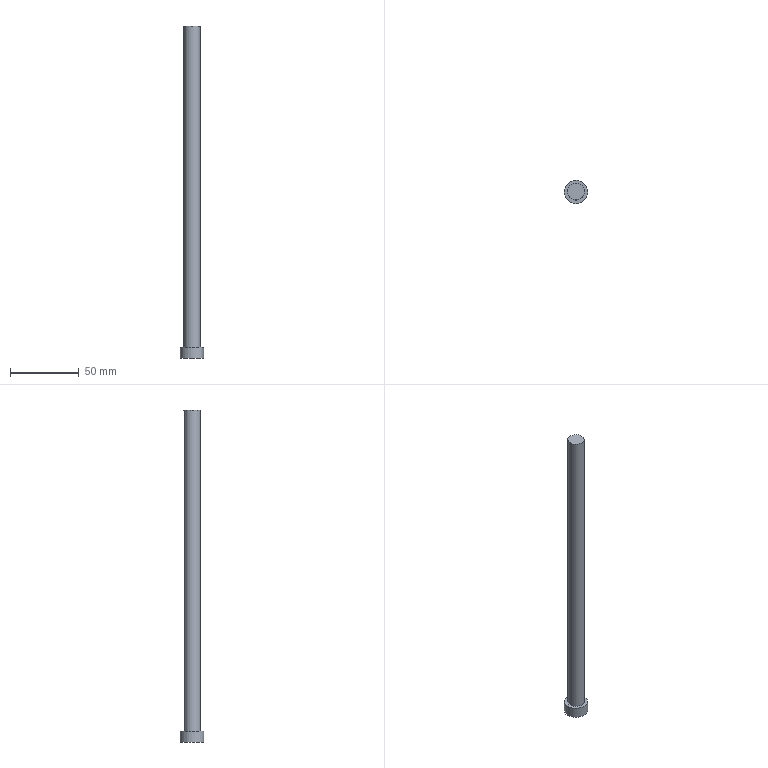Part | NX | features 模具.stp<1>[107] 2 | 1 solid | 5 faces | box 17 x 17 x 241.5 mm | volume 28224 mm3 | plane 3 | cylinder 2 | commonest cylinder face diameters 12 x1 17 x1
STEP:
#1=CARTESIAN_POINT('',(63.,0.,26.));
#2=VERTEX_POINT('',#1);
#3=CARTESIAN_POINT('',(69.,0.,26.));
#4=DIRECTION('',(0.,0.,-1.));
#5=DIRECTION('',(-1.,0.,0.));
#6=AXIS2_PLACEMENT_3D('',#3,#4,#5);
#7=CIRCLE('',#6,6.);
#8=EDGE_CURVE('',#2,#2,#7,.T.);
#9=ORIENTED_EDGE('',*,*,#8,.F.);
#10=EDGE_LOOP('',(#9));
#11=FACE_BOUND('',#10,.T.);
#12=CARTESIAN_POINT('',(-46.,0.,26.));
#13=DIRECTION('',(0.,0.,-1.));
#14=DIRECTION('',(0.,-1.,0.));
#15=AXIS2_PLACEMENT_3D('',#12,#13,#14);
#16=PLANE('',#15);
#17=ADVANCED_FACE('',(#11),#16,.F.);
#18=CARTESIAN_POINT('',(77.5,0.,-215.5));
#19=VERTEX_POINT('',#18);
#20=CARTESIAN_POINT('',(69.,0.,-215.5));
#21=DIRECTION('',(0.,0.,1.));
#22=DIRECTION('',(1.,0.,0.));
#23=AXIS2_PLACEMENT_3D('',#20,#21,#22);
#24=CIRCLE('',#23,8.5);
#25=EDGE_CURVE('',#19,#19,#24,.T.);
#26=ORIENTED_EDGE('',*,*,#25,.T.);
#27=EDGE_LOOP('',(#26));
#28=FACE_BOUND('',#27,.T.);
#29=CARTESIAN_POINT('',(77.5,0.,-207.5));
#30=VERTEX_POINT('',#29);
#31=CARTESIAN_POINT('',(69.,0.,-207.5));
#32=DIRECTION('',(0.,0.,-1.));
#33=DIRECTION('',(1.,0.,0.));
#34=AXIS2_PLACEMENT_3D('',#31,#32,#33);
#35=CIRCLE('',#34,8.5);
#36=EDGE_CURVE('',#30,#30,#35,.T.);
#37=ORIENTED_EDGE('',*,*,#36,.T.);
#38=EDGE_LOOP('',(#37));
#39=FACE_BOUND('',#38,.T.);
#40=CARTESIAN_POINT('',(69.,0.,-215.5));
#41=DIRECTION('',(0.,0.,1.));
#42=DIRECTION('',(1.,0.,0.));
#43=AXIS2_PLACEMENT_3D('',#40,#41,#42);
#44=CYLINDRICAL_SURFACE('',#43,8.5);
#45=ADVANCED_FACE('',(#28,#39),#44,.T.);
#46=ORIENTED_EDGE('',*,*,#25,.F.);
#47=EDGE_LOOP('',(#46));
#48=FACE_BOUND('',#47,.T.);
#49=CARTESIAN_POINT('',(69.,0.,-215.5));
#50=DIRECTION('',(0.,0.,-1.));
#51=DIRECTION('',(0.,-1.,0.));
#52=AXIS2_PLACEMENT_3D('',#49,#50,#51);
#53=PLANE('',#52);
#54=ADVANCED_FACE('',(#48),#53,.T.);
#55=ORIENTED_EDGE('',*,*,#36,.F.);
#56=EDGE_LOOP('',(#55));
#57=FACE_BOUND('',#56,.T.);
#58=CARTESIAN_POINT('',(75.,0.,-207.5));
#59=VERTEX_POINT('',#58);
#60=CARTESIAN_POINT('',(69.,0.,-207.5));
#61=DIRECTION('',(0.,0.,1.));
#62=DIRECTION('',(1.,0.,0.));
#63=AXIS2_PLACEMENT_3D('',#60,#61,#62);
#64=CIRCLE('',#63,6.);
#65=EDGE_CURVE('',#59,#59,#64,.T.);
#66=ORIENTED_EDGE('',*,*,#65,.F.);
#67=EDGE_LOOP('',(#66));
#68=FACE_BOUND('',#67,.T.);
#69=CARTESIAN_POINT('',(69.,0.,-207.5));
#70=DIRECTION('',(0.,0.,1.));
#71=DIRECTION('',(1.,0.,0.));
#72=AXIS2_PLACEMENT_3D('',#69,#70,#71);
#73=PLANE('',#72);
#74=ADVANCED_FACE('',(#57,#68),#73,.T.);
#75=ORIENTED_EDGE('',*,*,#8,.T.);
#76=EDGE_LOOP('',(#75));
#77=FACE_BOUND('',#76,.T.);
#78=ORIENTED_EDGE('',*,*,#65,.T.);
#79=EDGE_LOOP('',(#78));
#80=FACE_BOUND('',#79,.T.);
#81=CARTESIAN_POINT('',(69.,0.,-215.5));
#82=DIRECTION('',(0.,0.,1.));
#83=DIRECTION('',(1.,0.,0.));
#84=AXIS2_PLACEMENT_3D('',#81,#82,#83);
#85=CYLINDRICAL_SURFACE('',#84,6.);
#86=ADVANCED_FACE('',(#77,#80),#85,.T.);
#87=CLOSED_SHELL('',(#17,#45,#54,#74,#86));
#88=MANIFOLD_SOLID_BREP('',#87);
#89=(LENGTH_UNIT()NAMED_UNIT(*)SI_UNIT(.MILLI.,.METRE.));
#90=UNCERTAINTY_MEASURE_WITH_UNIT(LENGTH_MEASURE(0.00001),#89,'','');
#91=(NAMED_UNIT(*)PLANE_ANGLE_UNIT()SI_UNIT($,.RADIAN.));
#92=(NAMED_UNIT(*)SI_UNIT($,.STERADIAN.)SOLID_ANGLE_UNIT());
#93=(GEOMETRIC_REPRESENTATION_CONTEXT(3)GLOBAL_UNCERTAINTY_ASSIGNED_CONTEXT((#90))GLOBAL_UNIT_ASSIGNED_CONTEXT((#89,#91,#92))REPRESENTATION_CONTEXT('',''));
#94=ADVANCED_BREP_SHAPE_REPRESENTATION('',(#88),#93);